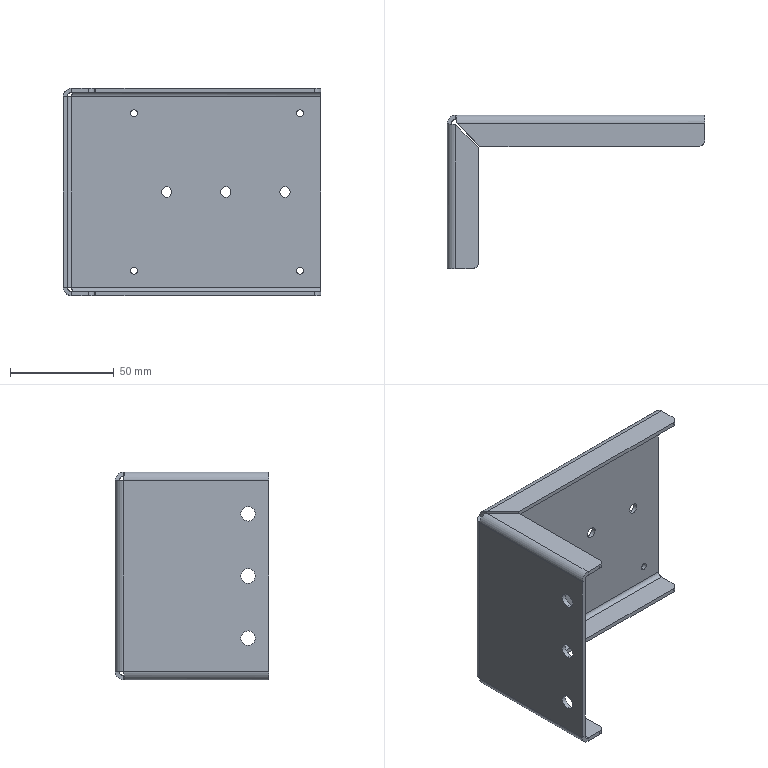Part | NX | features BREP 1 | 1 solid | 70 faces | box 124 x 74 x 100 mm | volume 46776 mm3 | cylinder 34 | plane 32 | spline 4 | commonest cylinder face diameters 3.3 x8 5 x6 7 x6 4 x5 8 x5 6 x4